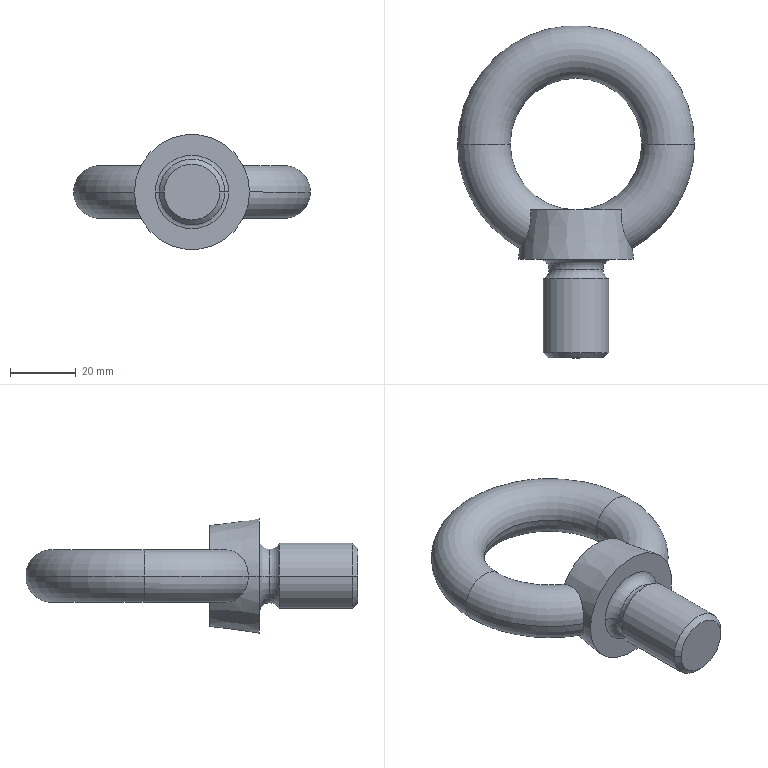Part | STEP file | SCHI20-Part-2 | 1 solid | 20 faces | box 72 x 101 x 35 mm | volume 51064 mm3 | torus 10 | cone 4 | plane 4 | cylinder 2 | commonest cylinder face diameters 20 x2